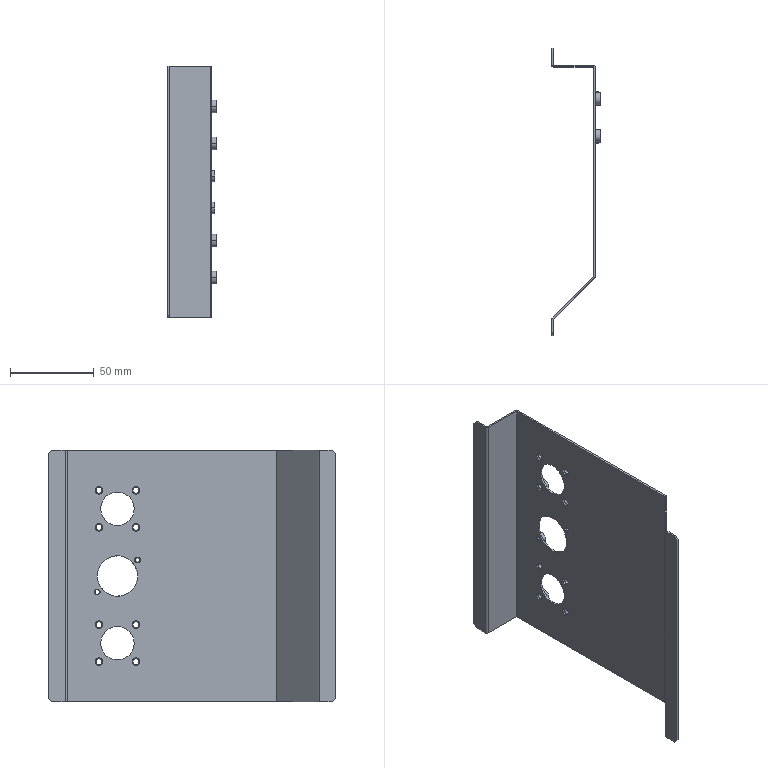Part | SolidWorks | features ICE 5, BossThin 2, Chamfer 1, MirrorPattern 1, SplitBody 1 | 1 solid | 133 faces | box 29 x 171 x 150 mm | volume 30583 mm3 | cylinder 74 | plane 59 | commonest cylinder face diameters 3.5 x20 4.5 x16 7.5 x16 0.2 x4 2.2 x4 2.8 x4